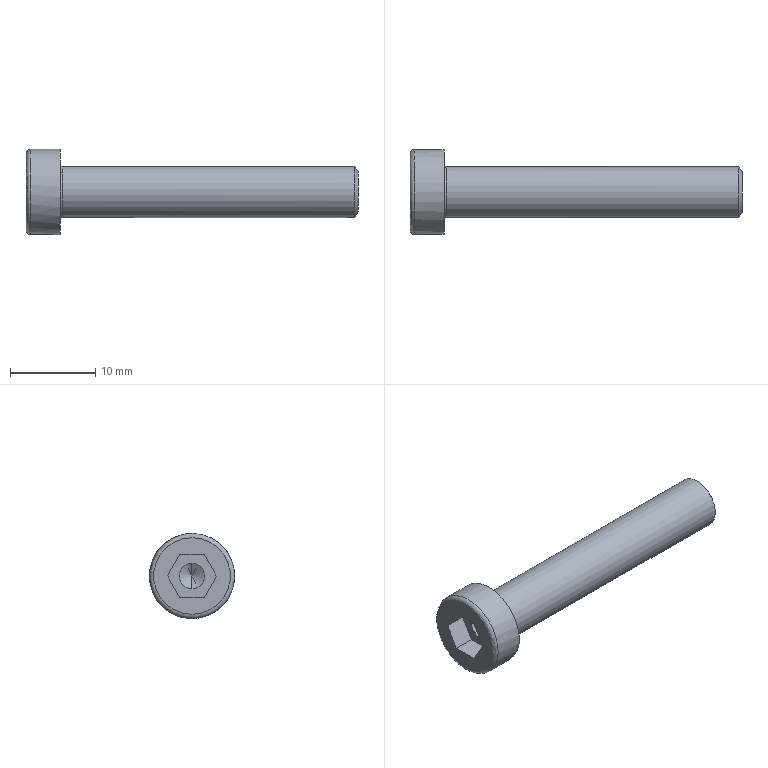Part | STEP file | Part [20] | 1 solid | 18 faces | box 39 x 10 x 10 mm | volume 1226 mm3 | plane 10 | cylinder 3 | cone 3 | torus 2 | commonest cylinder face diameters 3 x1 6 x1 10 x1
STEP:
#1=CARTESIAN_POINT('',(-20.293,107.5,4.5));
#2=VERTEX_POINT('',#1);
#3=CARTESIAN_POINT('',(-20.293,107.5,0.));
#4=DIRECTION('',(-1.,0.,0.));
#5=DIRECTION('',(0.,0.,1.));
#6=AXIS2_PLACEMENT_3D('',#3,#4,#5);
#7=CIRCLE('',#6,4.5);
#8=EDGE_CURVE('',#2,#2,#7,.T.);
#9=ORIENTED_EDGE('',*,*,#8,.T.);
#10=EDGE_LOOP('',(#9));
#11=FACE_BOUND('',#10,.T.);
#12=CARTESIAN_POINT('',(-20.293,108.948,-2.497));
#13=VERTEX_POINT('',#12);
#14=CARTESIAN_POINT('',(-20.293,110.387,0.005038));
#15=VERTEX_POINT('',#14);
#16=CARTESIAN_POINT('',(-20.293,108.948,-2.497));
#17=DIRECTION('',(0.,0.4985,0.8669));
#18=VECTOR('',#17,1.);
#19=LINE('',#16,#18);
#20=EDGE_CURVE('',#13,#15,#19,.T.);
#21=ORIENTED_EDGE('',*,*,#20,.T.);
#22=CARTESIAN_POINT('',(-20.293,108.939,2.503));
#23=VERTEX_POINT('',#22);
#24=CARTESIAN_POINT('',(-20.293,110.387,0.005038));
#25=DIRECTION('',(0.,-0.5015,0.8652));
#26=VECTOR('',#25,1.);
#27=LINE('',#24,#26);
#28=EDGE_CURVE('',#15,#23,#27,.T.);
#29=ORIENTED_EDGE('',*,*,#28,.T.);
#30=CARTESIAN_POINT('',(-20.293,106.052,2.497));
#31=VERTEX_POINT('',#30);
#32=CARTESIAN_POINT('',(-20.293,108.939,2.503));
#33=DIRECTION('',(0.,-1.,-0.001745));
#34=VECTOR('',#33,1.);
#35=LINE('',#32,#34);
#36=EDGE_CURVE('',#23,#31,#35,.T.);
#37=ORIENTED_EDGE('',*,*,#36,.T.);
#38=CARTESIAN_POINT('',(-20.293,104.613,-0.005038));
#39=VERTEX_POINT('',#38);
#40=CARTESIAN_POINT('',(-20.293,106.052,2.497));
#41=DIRECTION('',(0.,-0.4985,-0.8669));
#42=VECTOR('',#41,1.);
#43=LINE('',#40,#42);
#44=EDGE_CURVE('',#31,#39,#43,.T.);
#45=ORIENTED_EDGE('',*,*,#44,.T.);
#46=CARTESIAN_POINT('',(-20.293,106.061,-2.503));
#47=VERTEX_POINT('',#46);
#48=CARTESIAN_POINT('',(-20.293,104.613,-0.005038));
#49=DIRECTION('',(0.,0.5015,-0.8652));
#50=VECTOR('',#49,1.);
#51=LINE('',#48,#50);
#52=EDGE_CURVE('',#39,#47,#51,.T.);
#53=ORIENTED_EDGE('',*,*,#52,.T.);
#54=CARTESIAN_POINT('',(-20.293,106.061,-2.503));
#55=DIRECTION('',(0.,1.,0.001745));
#56=VECTOR('',#55,1.);
#57=LINE('',#54,#56);
#58=EDGE_CURVE('',#47,#13,#57,.T.);
#59=ORIENTED_EDGE('',*,*,#58,.T.);
#60=EDGE_LOOP('',(#21,#29,#37,#45,#53,#59));
#61=FACE_BOUND('',#60,.T.);
#62=CARTESIAN_POINT('',(-20.293,107.5,0.));
#63=DIRECTION('',(1.,0.,0.));
#64=DIRECTION('',(0.,0.,1.));
#65=AXIS2_PLACEMENT_3D('',#62,#63,#64);
#66=PLANE('',#65);
#67=ADVANCED_FACE('',(#11,#61),#66,.F.);
#68=CARTESIAN_POINT('',(-19.793,107.5,5.));
#69=VERTEX_POINT('',#68);
#70=CARTESIAN_POINT('',(-19.793,107.5,5.));
#71=CARTESIAN_POINT('',(-19.793,107.395,5.));
#72=CARTESIAN_POINT('',(-19.793,107.186,4.993));
#73=CARTESIAN_POINT('',(-19.793,106.873,4.964));
#74=CARTESIAN_POINT('',(-19.793,106.562,4.915));
#75=CARTESIAN_POINT('',(-19.793,106.256,4.846));
#76=CARTESIAN_POINT('',(-19.793,105.954,4.758));
#77=CARTESIAN_POINT('',(-19.793,105.658,4.652));
#78=CARTESIAN_POINT('',(-19.793,105.369,4.527));
#79=CARTESIAN_POINT('',(-19.793,105.089,4.384));
#80=CARTESIAN_POINT('',(-19.793,104.819,4.224));
#81=CARTESIAN_POINT('',(-19.793,104.559,4.047));
#82=CARTESIAN_POINT('',(-19.793,104.31,3.855));
#83=CARTESIAN_POINT('',(-19.793,104.075,3.647));
#84=CARTESIAN_POINT('',(-19.793,103.852,3.425));
#85=CARTESIAN_POINT('',(-19.793,103.644,3.189));
#86=CARTESIAN_POINT('',(-19.793,103.452,2.94));
#87=CARTESIAN_POINT('',(-19.793,103.275,2.68));
#88=CARTESIAN_POINT('',(-19.793,103.115,2.41));
#89=CARTESIAN_POINT('',(-19.793,102.973,2.129));
#90=CARTESIAN_POINT('',(-19.793,102.848,1.841));
#91=CARTESIAN_POINT('',(-19.793,102.741,1.545));
#92=CARTESIAN_POINT('',(-19.793,102.654,1.243));
#93=CARTESIAN_POINT('',(-19.793,102.585,0.9364));
#94=CARTESIAN_POINT('',(-19.793,102.536,0.6259));
#95=CARTESIAN_POINT('',(-19.793,102.507,0.313));
#96=CARTESIAN_POINT('',(-19.793,102.497,-0.001251));
#97=CARTESIAN_POINT('',(-19.793,102.507,-0.3155));
#98=CARTESIAN_POINT('',(-19.793,102.536,-0.6284));
#99=CARTESIAN_POINT('',(-19.793,102.586,-0.9389));
#100=CARTESIAN_POINT('',(-19.793,102.654,-1.246));
#101=CARTESIAN_POINT('',(-19.793,102.742,-1.548));
#102=CARTESIAN_POINT('',(-19.793,102.849,-1.843));
#103=CARTESIAN_POINT('',(-19.793,102.974,-2.132));
#104=CARTESIAN_POINT('',(-19.793,103.116,-2.412));
#105=CARTESIAN_POINT('',(-19.793,103.276,-2.682));
#106=CARTESIAN_POINT('',(-19.793,103.453,-2.942));
#107=CARTESIAN_POINT('',(-19.793,103.646,-3.191));
#108=CARTESIAN_POINT('',(-19.793,103.854,-3.426));
#109=CARTESIAN_POINT('',(-19.793,104.076,-3.649));
#110=CARTESIAN_POINT('',(-19.793,104.312,-3.856));
#111=CARTESIAN_POINT('',(-19.793,104.561,-4.049));
#112=CARTESIAN_POINT('',(-19.793,104.821,-4.226));
#113=CARTESIAN_POINT('',(-19.793,105.091,-4.385));
#114=CARTESIAN_POINT('',(-19.793,105.372,-4.528));
#115=CARTESIAN_POINT('',(-19.793,105.66,-4.653));
#116=CARTESIAN_POINT('',(-19.793,105.956,-4.759));
#117=CARTESIAN_POINT('',(-19.793,106.258,-4.847));
#118=CARTESIAN_POINT('',(-19.793,106.565,-4.915));
#119=CARTESIAN_POINT('',(-19.793,106.875,-4.964));
#120=CARTESIAN_POINT('',(-19.793,107.187,-4.993));
#121=CARTESIAN_POINT('',(-19.793,107.396,-5.));
#122=CARTESIAN_POINT('',(-19.793,107.5,-5.));
#123=CARTESIAN_POINT('',(-19.793,107.605,-5.));
#124=CARTESIAN_POINT('',(-19.793,107.814,-4.993));
#125=CARTESIAN_POINT('',(-19.793,108.127,-4.964));
#126=CARTESIAN_POINT('',(-19.793,108.438,-4.915));
#127=CARTESIAN_POINT('',(-19.793,108.744,-4.846));
#128=CARTESIAN_POINT('',(-19.793,109.046,-4.758));
#129=CARTESIAN_POINT('',(-19.793,109.342,-4.652));
#130=CARTESIAN_POINT('',(-19.793,109.631,-4.527));
#131=CARTESIAN_POINT('',(-19.793,109.911,-4.384));
#132=CARTESIAN_POINT('',(-19.793,110.181,-4.224));
#133=CARTESIAN_POINT('',(-19.793,110.441,-4.047));
#134=CARTESIAN_POINT('',(-19.793,110.69,-3.855));
#135=CARTESIAN_POINT('',(-19.793,110.925,-3.647));
#136=CARTESIAN_POINT('',(-19.793,111.148,-3.425));
#137=CARTESIAN_POINT('',(-19.793,111.356,-3.189));
#138=CARTESIAN_POINT('',(-19.793,111.548,-2.94));
#139=CARTESIAN_POINT('',(-19.793,111.725,-2.68));
#140=CARTESIAN_POINT('',(-19.793,111.885,-2.41));
#141=CARTESIAN_POINT('',(-19.793,112.027,-2.129));
#142=CARTESIAN_POINT('',(-19.793,112.152,-1.841));
#143=CARTESIAN_POINT('',(-19.793,112.259,-1.545));
#144=CARTESIAN_POINT('',(-19.793,112.346,-1.243));
#145=CARTESIAN_POINT('',(-19.793,112.415,-0.9364));
#146=CARTESIAN_POINT('',(-19.793,112.464,-0.6259));
#147=CARTESIAN_POINT('',(-19.793,112.493,-0.313));
#148=CARTESIAN_POINT('',(-19.793,112.503,0.001251));
#149=CARTESIAN_POINT('',(-19.793,112.493,0.3155));
#150=CARTESIAN_POINT('',(-19.793,112.464,0.6284));
#151=CARTESIAN_POINT('',(-19.793,112.414,0.9389));
#152=CARTESIAN_POINT('',(-19.793,112.346,1.246));
#153=CARTESIAN_POINT('',(-19.793,112.258,1.548));
#154=CARTESIAN_POINT('',(-19.793,112.151,1.843));
#155=CARTESIAN_POINT('',(-19.793,112.026,2.132));
#156=CARTESIAN_POINT('',(-19.793,111.884,2.412));
#157=CARTESIAN_POINT('',(-19.793,111.724,2.682));
#158=CARTESIAN_POINT('',(-19.793,111.547,2.942));
#159=CARTESIAN_POINT('',(-19.793,111.354,3.191));
#160=CARTESIAN_POINT('',(-19.793,111.146,3.426));
#161=CARTESIAN_POINT('',(-19.793,110.924,3.649));
#162=CARTESIAN_POINT('',(-19.793,110.688,3.856));
#163=CARTESIAN_POINT('',(-19.793,110.439,4.049));
#164=CARTESIAN_POINT('',(-19.793,110.179,4.226));
#165=CARTESIAN_POINT('',(-19.793,109.909,4.385));
#166=CARTESIAN_POINT('',(-19.793,109.628,4.528));
#167=CARTESIAN_POINT('',(-19.793,109.34,4.653));
#168=CARTESIAN_POINT('',(-19.793,109.044,4.759));
#169=CARTESIAN_POINT('',(-19.793,108.742,4.847));
#170=CARTESIAN_POINT('',(-19.793,108.435,4.915));
#171=CARTESIAN_POINT('',(-19.793,108.125,4.964));
#172=CARTESIAN_POINT('',(-19.793,107.813,4.993));
#173=CARTESIAN_POINT('',(-19.793,107.604,5.));
#174=CARTESIAN_POINT('',(-19.793,107.5,5.));
#175=B_SPLINE_CURVE_WITH_KNOTS('',3,(#70,#71,#72,#73,#74,#75,#76,#77,#78,#79,#80,#81,#82,#83,#84,#85,#86,#87,#88,#89,#90,#91,#92,#93,#94,#95,#96,#97,#98,#99,#100,#101,#102,#103,#104,#105,#106,#107,#108,#109,#110,#111,#112,#113,#114,#115,#116,#117,#118,#119,#120,#121,#122,#123,#124,#125,#126,#127,#128,#129,#130,#131,#132,#133,#134,#135,#136,#137,#138,#139,#140,#141,#142,#143,#144,#145,#146,#147,#148,#149,#150,#151,#152,#153,#154,#155,#156,#157,#158,#159,#160,#161,#162,#163,#164,#165,#166,#167,#168,#169,#170,#171,#172,#173,#174),.UNSPECIFIED.,.T.,.F.,(4,1,1,1,1,1,1,1,1,1,1,1,1,1,1,1,1,1,1,1,1,1,1,1,1,1,1,1,1,1,1,1,1,1,1,1,1,1,1,1,1,1,1,1,1,1,1,1,1,1,3,1,1,1,1,1,1,1,1,1,1,1,1,1,1,1,1,1,1,1,1,1,1,1,1,1,1,1,1,1,1,1,1,1,1,1,1,1,1,1,1,1,1,1,1,1,1,1,1,1,4),(0.,0.01,0.02,0.03,0.04001,0.05001,0.06001,0.07001,0.08001,0.09001,0.1,0.11,0.12,0.13,0.14,0.15,0.16,0.17,0.18,0.19,0.2,0.21,0.22,0.23,0.24,0.25,0.26,0.27,0.28,0.29,0.3,0.31,0.3201,0.3301,0.3401,0.3501,0.3601,0.3701,0.3801,0.3901,0.4001,0.4101,0.4201,0.4301,0.4401,0.4501,0.4601,0.4701,0.4801,0.4901,0.5,0.51,0.52,0.53,0.54,0.55,0.56,0.57,0.58,0.59,0.6,0.61,0.62,0.63,0.64,0.65,0.66,0.67,0.68,0.69,0.7,0.71,0.72,0.73,0.74,0.75,0.76,0.77,0.78,0.79,0.8,0.81,0.8201,0.8301,0.8401,0.8501,0.8601,0.8701,0.8801,0.8901,0.9001,0.9101,0.9201,0.9301,0.9401,0.9501,0.9601,0.9701,0.9801,0.9901,1.),.UNSPECIFIED.);
#176=EDGE_CURVE('',#69,#69,#175,.T.);
#177=ORIENTED_EDGE('',*,*,#176,.F.);
#178=EDGE_LOOP('',(#177));
#179=FACE_OUTER_BOUND('',#178,.T.);
#180=ORIENTED_EDGE('',*,*,#8,.F.);
#181=EDGE_LOOP('',(#180));
#182=FACE_OUTER_BOUND('',#181,.T.);
#183=CARTESIAN_POINT('',(-19.793,107.5,0.));
#184=DIRECTION('',(1.,0.,0.));
#185=DIRECTION('',(0.,0.,1.));
#186=AXIS2_PLACEMENT_3D('',#183,#184,#185);
#187=TOROIDAL_SURFACE('',#186,4.5,0.5);
#188=ADVANCED_FACE('',(#179,#182),#187,.T.);
#189=CARTESIAN_POINT('',(-16.293,107.5,5.));
#190=VERTEX_POINT('',#189);
#191=CARTESIAN_POINT('',(-16.293,107.5,0.));
#192=DIRECTION('',(1.,0.,0.));
#193=DIRECTION('',(0.,0.,1.));
#194=AXIS2_PLACEMENT_3D('',#191,#192,#193);
#195=CIRCLE('',#194,5.);
#196=EDGE_CURVE('',#190,#190,#195,.T.);
#197=ORIENTED_EDGE('',*,*,#196,.F.);
#198=EDGE_LOOP('',(#197));
#199=FACE_OUTER_BOUND('',#198,.T.);
#200=ORIENTED_EDGE('',*,*,#176,.T.);
#201=EDGE_LOOP('',(#200));
#202=FACE_OUTER_BOUND('',#201,.T.);
#203=CARTESIAN_POINT('',(-22.243,107.5,0.));
#204=DIRECTION('',(1.,0.,0.));
#205=DIRECTION('',(0.,0.,1.));
#206=AXIS2_PLACEMENT_3D('',#203,#204,#205);
#207=CYLINDRICAL_SURFACE('',#206,5.);
#208=ADVANCED_FACE('',(#199,#202),#207,.T.);
#209=ORIENTED_EDGE('',*,*,#196,.T.);
#210=EDGE_LOOP('',(#209));
#211=FACE_BOUND('',#210,.T.);
#212=CARTESIAN_POINT('',(-16.293,107.5,3.25));
#213=VERTEX_POINT('',#212);
#214=CARTESIAN_POINT('',(-16.293,107.5,0.));
#215=DIRECTION('',(1.,0.,0.));
#216=DIRECTION('',(0.,0.,1.));
#217=AXIS2_PLACEMENT_3D('',#214,#215,#216);
#218=CIRCLE('',#217,3.25);
#219=EDGE_CURVE('',#213,#213,#218,.T.);
#220=ORIENTED_EDGE('',*,*,#219,.F.);
#221=EDGE_LOOP('',(#220));
#222=FACE_BOUND('',#221,.T.);
#223=CARTESIAN_POINT('',(-16.293,107.5,0.));
#224=DIRECTION('',(1.,0.,0.));
#225=DIRECTION('',(0.,0.,1.));
#226=AXIS2_PLACEMENT_3D('',#223,#224,#225);
#227=PLANE('',#226);
#228=ADVANCED_FACE('',(#211,#222),#227,.T.);
#229=CARTESIAN_POINT('',(-16.043,107.5,3.));
#230=VERTEX_POINT('',#229);
#231=CARTESIAN_POINT('',(-16.043,107.5,3.));
#232=CARTESIAN_POINT('',(-16.043,107.437,3.));
#233=CARTESIAN_POINT('',(-16.043,107.311,2.996));
#234=CARTESIAN_POINT('',(-16.043,107.124,2.978));
#235=CARTESIAN_POINT('',(-16.043,106.937,2.949));
#236=CARTESIAN_POINT('',(-16.043,106.753,2.908));
#237=CARTESIAN_POINT('',(-16.043,106.572,2.855));
#238=CARTESIAN_POINT('',(-16.043,106.395,2.791));
#239=CARTESIAN_POINT('',(-16.043,106.222,2.716));
#240=CARTESIAN_POINT('',(-16.043,106.054,2.631));
#241=CARTESIAN_POINT('',(-16.043,105.891,2.535));
#242=CARTESIAN_POINT('',(-16.043,105.735,2.428));
#243=CARTESIAN_POINT('',(-16.043,105.586,2.313));
#244=CARTESIAN_POINT('',(-16.043,105.445,2.188));
#245=CARTESIAN_POINT('',(-16.043,105.311,2.055));
#246=CARTESIAN_POINT('',(-16.043,105.187,1.913));
#247=CARTESIAN_POINT('',(-16.043,105.071,1.764));
#248=CARTESIAN_POINT('',(-16.043,104.965,1.608));
#249=CARTESIAN_POINT('',(-16.043,104.869,1.446));
#250=CARTESIAN_POINT('',(-16.043,104.784,1.278));
#251=CARTESIAN_POINT('',(-16.043,104.709,1.105));
#252=CARTESIAN_POINT('',(-16.043,104.645,0.9271));
#253=CARTESIAN_POINT('',(-16.043,104.592,0.746));
#254=CARTESIAN_POINT('',(-16.043,104.551,0.5619));
#255=CARTESIAN_POINT('',(-16.043,104.522,0.3756));
#256=CARTESIAN_POINT('',(-16.043,104.504,0.1878));
#257=CARTESIAN_POINT('',(-16.043,104.498,-0.0007505));
#258=CARTESIAN_POINT('',(-16.043,104.504,-0.1893));
#259=CARTESIAN_POINT('',(-16.043,104.522,-0.3771));
#260=CARTESIAN_POINT('',(-16.043,104.551,-0.5633));
#261=CARTESIAN_POINT('',(-16.043,104.593,-0.7474));
#262=CARTESIAN_POINT('',(-16.043,104.645,-0.9285));
#263=CARTESIAN_POINT('',(-16.043,104.709,-1.106));
#264=CARTESIAN_POINT('',(-16.043,104.784,-1.279));
#265=CARTESIAN_POINT('',(-16.043,104.87,-1.447));
#266=CARTESIAN_POINT('',(-16.043,104.966,-1.609));
#267=CARTESIAN_POINT('',(-16.043,105.072,-1.765));
#268=CARTESIAN_POINT('',(-16.043,105.188,-1.914));
#269=CARTESIAN_POINT('',(-16.043,105.312,-2.056));
#270=CARTESIAN_POINT('',(-16.043,105.446,-2.189));
#271=CARTESIAN_POINT('',(-16.043,105.587,-2.314));
#272=CARTESIAN_POINT('',(-16.043,105.736,-2.429));
#273=CARTESIAN_POINT('',(-16.043,105.893,-2.535));
#274=CARTESIAN_POINT('',(-16.043,106.055,-2.631));
#275=CARTESIAN_POINT('',(-16.043,106.223,-2.717));
#276=CARTESIAN_POINT('',(-16.043,106.396,-2.792));
#277=CARTESIAN_POINT('',(-16.043,106.574,-2.855));
#278=CARTESIAN_POINT('',(-16.043,106.755,-2.908));
#279=CARTESIAN_POINT('',(-16.043,106.939,-2.949));
#280=CARTESIAN_POINT('',(-16.043,107.125,-2.978));
#281=CARTESIAN_POINT('',(-16.043,107.312,-2.996));
#282=CARTESIAN_POINT('',(-16.043,107.438,-3.));
#283=CARTESIAN_POINT('',(-16.043,107.5,-3.));
#284=CARTESIAN_POINT('',(-16.043,107.563,-3.));
#285=CARTESIAN_POINT('',(-16.043,107.689,-2.996));
#286=CARTESIAN_POINT('',(-16.043,107.876,-2.978));
#287=CARTESIAN_POINT('',(-16.043,108.063,-2.949));
#288=CARTESIAN_POINT('',(-16.043,108.247,-2.908));
#289=CARTESIAN_POINT('',(-16.043,108.428,-2.855));
#290=CARTESIAN_POINT('',(-16.043,108.605,-2.791));
#291=CARTESIAN_POINT('',(-16.043,108.778,-2.716));
#292=CARTESIAN_POINT('',(-16.043,108.946,-2.631));
#293=CARTESIAN_POINT('',(-16.043,109.109,-2.535));
#294=CARTESIAN_POINT('',(-16.043,109.265,-2.428));
#295=CARTESIAN_POINT('',(-16.043,109.414,-2.313));
#296=CARTESIAN_POINT('',(-16.043,109.555,-2.188));
#297=CARTESIAN_POINT('',(-16.043,109.689,-2.055));
#298=CARTESIAN_POINT('',(-16.043,109.813,-1.913));
#299=CARTESIAN_POINT('',(-16.043,109.929,-1.764));
#300=CARTESIAN_POINT('',(-16.043,110.035,-1.608));
#301=CARTESIAN_POINT('',(-16.043,110.131,-1.446));
#302=CARTESIAN_POINT('',(-16.043,110.216,-1.278));
#303=CARTESIAN_POINT('',(-16.043,110.291,-1.105));
#304=CARTESIAN_POINT('',(-16.043,110.355,-0.9271));
#305=CARTESIAN_POINT('',(-16.043,110.408,-0.746));
#306=CARTESIAN_POINT('',(-16.043,110.449,-0.5619));
#307=CARTESIAN_POINT('',(-16.043,110.478,-0.3756));
#308=CARTESIAN_POINT('',(-16.043,110.496,-0.1878));
#309=CARTESIAN_POINT('',(-16.043,110.502,0.0007505));
#310=CARTESIAN_POINT('',(-16.043,110.496,0.1893));
#311=CARTESIAN_POINT('',(-16.043,110.478,0.3771));
#312=CARTESIAN_POINT('',(-16.043,110.449,0.5633));
#313=CARTESIAN_POINT('',(-16.043,110.407,0.7474));
#314=CARTESIAN_POINT('',(-16.043,110.355,0.9285));
#315=CARTESIAN_POINT('',(-16.043,110.291,1.106));
#316=CARTESIAN_POINT('',(-16.043,110.216,1.279));
#317=CARTESIAN_POINT('',(-16.043,110.13,1.447));
#318=CARTESIAN_POINT('',(-16.043,110.034,1.609));
#319=CARTESIAN_POINT('',(-16.043,109.928,1.765));
#320=CARTESIAN_POINT('',(-16.043,109.812,1.914));
#321=CARTESIAN_POINT('',(-16.043,109.688,2.056));
#322=CARTESIAN_POINT('',(-16.043,109.554,2.189));
#323=CARTESIAN_POINT('',(-16.043,109.413,2.314));
#324=CARTESIAN_POINT('',(-16.043,109.264,2.429));
#325=CARTESIAN_POINT('',(-16.043,109.107,2.535));
#326=CARTESIAN_POINT('',(-16.043,108.945,2.631));
#327=CARTESIAN_POINT('',(-16.043,108.777,2.717));
#328=CARTESIAN_POINT('',(-16.043,108.604,2.792));
#329=CARTESIAN_POINT('',(-16.043,108.426,2.855));
#330=CARTESIAN_POINT('',(-16.043,108.245,2.908));
#331=CARTESIAN_POINT('',(-16.043,108.061,2.949));
#332=CARTESIAN_POINT('',(-16.043,107.875,2.978));
#333=CARTESIAN_POINT('',(-16.043,107.688,2.996));
#334=CARTESIAN_POINT('',(-16.043,107.562,3.));
#335=CARTESIAN_POINT('',(-16.043,107.5,3.));
#336=B_SPLINE_CURVE_WITH_KNOTS('',3,(#231,#232,#233,#234,#235,#236,#237,#238,#239,#240,#241,#242,#243,#244,#245,#246,#247,#248,#249,#250,#251,#252,#253,#254,#255,#256,#257,#258,#259,#260,#261,#262,#263,#264,#265,#266,#267,#268,#269,#270,#271,#272,#273,#274,#275,#276,#277,#278,#279,#280,#281,#282,#283,#284,#285,#286,#287,#288,#289,#290,#291,#292,#293,#294,#295,#296,#297,#298,#299,#300,#301,#302,#303,#304,#305,#306,#307,#308,#309,#310,#311,#312,#313,#314,#315,#316,#317,#318,#319,#320,#321,#322,#323,#324,#325,#326,#327,#328,#329,#330,#331,#332,#333,#334,#335),.UNSPECIFIED.,.T.,.F.,(4,1,1,1,1,1,1,1,1,1,1,1,1,1,1,1,1,1,1,1,1,1,1,1,1,1,1,1,1,1,1,1,1,1,1,1,1,1,1,1,1,1,1,1,1,1,1,1,1,1,3,1,1,1,1,1,1,1,1,1,1,1,1,1,1,1,1,1,1,1,1,1,1,1,1,1,1,1,1,1,1,1,1,1,1,1,1,1,1,1,1,1,1,1,1,1,1,1,1,1,4),(0.,0.01,0.02,0.03,0.04001,0.05001,0.06001,0.07001,0.08001,0.09001,0.1,0.11,0.12,0.13,0.14,0.15,0.16,0.17,0.18,0.19,0.2,0.21,0.22,0.23,0.24,0.25,0.26,0.27,0.28,0.29,0.3,0.31,0.3201,0.3301,0.3401,0.3501,0.3601,0.3701,0.3801,0.3901,0.4001,0.4101,0.4201,0.4301,0.4401,0.4501,0.4601,0.4701,0.4801,0.4901,0.5,0.51,0.52,0.53,0.54,0.55,0.56,0.57,0.58,0.59,0.6,0.61,0.62,0.63,0.64,0.65,0.66,0.67,0.68,0.69,0.7,0.71,0.72,0.73,0.74,0.75,0.76,0.77,0.78,0.79,0.8,0.81,0.8201,0.8301,0.8401,0.8501,0.8601,0.8701,0.8801,0.8901,0.9001,0.9101,0.9201,0.9301,0.9401,0.9501,0.9601,0.9701,0.9801,0.9901,1.),.UNSPECIFIED.);
#337=EDGE_CURVE('',#230,#230,#336,.T.);
#338=ORIENTED_EDGE('',*,*,#337,.F.);
#339=EDGE_LOOP('',(#338));
#340=FACE_OUTER_BOUND('',#339,.T.);
#341=ORIENTED_EDGE('',*,*,#219,.T.);
#342=EDGE_LOOP('',(#341));
#343=FACE_OUTER_BOUND('',#342,.T.);
#344=CARTESIAN_POINT('',(-16.043,107.5,0.));
#345=DIRECTION('',(1.,0.,0.));
#346=DIRECTION('',(0.,0.,1.));
#347=AXIS2_PLACEMENT_3D('',#344,#345,#346);
#348=TOROIDAL_SURFACE('',#347,3.25,0.25);
#349=ADVANCED_FACE('',(#340,#343),#348,.F.);
#350=CARTESIAN_POINT('',(18.273,107.5,3.));
#351=VERTEX_POINT('',#350);
#352=CARTESIAN_POINT('',(18.273,107.5,-3.));
#353=VERTEX_POINT('',#352);
#354=CARTESIAN_POINT('',(18.273,107.5,0.));
#355=DIRECTION('',(-1.,0.,0.));
#356=DIRECTION('',(0.,0.,1.));
#357=AXIS2_PLACEMENT_3D('',#354,#355,#356);
#358=CIRCLE('',#357,3.);
#359=EDGE_CURVE('',#351,#353,#358,.T.);
#360=ORIENTED_EDGE('',*,*,#359,.T.);
#361=CARTESIAN_POINT('',(18.273,107.5,0.));
#362=DIRECTION('',(1.,0.,0.));
#363=DIRECTION('',(0.,0.,1.));
#364=AXIS2_PLACEMENT_3D('',#361,#362,#363);
#365=CIRCLE('',#364,3.);
#366=EDGE_CURVE('',#351,#353,#365,.T.);
#367=ORIENTED_EDGE('',*,*,#366,.F.);
#368=EDGE_LOOP('',(#360,#367));
#369=FACE_BOUND('',#368,.T.);
#370=ORIENTED_EDGE('',*,*,#337,.T.);
#371=EDGE_LOOP('',(#370));
#372=FACE_OUTER_BOUND('',#371,.T.);
#373=CARTESIAN_POINT('',(-22.243,107.5,0.));
#374=DIRECTION('',(1.,0.,0.));
#375=DIRECTION('',(0.,0.,1.));
#376=AXIS2_PLACEMENT_3D('',#373,#374,#375);
#377=CYLINDRICAL_SURFACE('',#376,3.);
#378=ADVANCED_FACE('',(#369,#372),#377,.T.);
#379=CARTESIAN_POINT('',(18.707,107.5,-2.386));
#380=VERTEX_POINT('',#379);
#381=CARTESIAN_POINT('',(18.707,107.5,0.));
#382=DIRECTION('',(1.,0.,0.));
#383=DIRECTION('',(0.,0.,1.));
#384=AXIS2_PLACEMENT_3D('',#381,#382,#383);
#385=CIRCLE('',#384,2.386);
#386=EDGE_CURVE('',#380,#380,#385,.T.);
#387=ORIENTED_EDGE('',*,*,#386,.F.);
#388=EDGE_LOOP('',(#387));
#389=FACE_OUTER_BOUND('',#388,.T.);
#390=ORIENTED_EDGE('',*,*,#366,.T.);
#391=ORIENTED_EDGE('',*,*,#359,.F.);
#392=EDGE_LOOP('',(#390,#391));
#393=FACE_BOUND('',#392,.T.);
#394=CARTESIAN_POINT('',(18.49,107.5,0.));
#395=DIRECTION('',(-1.,0.,0.));
#396=DIRECTION('',(0.,0.,-1.));
#397=AXIS2_PLACEMENT_3D('',#394,#395,#396);
#398=CONICAL_SURFACE('',#397,2.693,0.9553);
#399=ADVANCED_FACE('',(#389,#393),#398,.T.);
#400=ORIENTED_EDGE('',*,*,#386,.T.);
#401=EDGE_LOOP('',(#400));
#402=FACE_BOUND('',#401,.T.);
#403=CARTESIAN_POINT('',(18.707,107.5,0.));
#404=DIRECTION('',(1.,0.,0.));
#405=DIRECTION('',(0.,0.,1.));
#406=AXIS2_PLACEMENT_3D('',#403,#404,#405);
#407=PLANE('',#406);
#408=ADVANCED_FACE('',(#402),#407,.T.);
#409=CARTESIAN_POINT('',(-17.793,106.061,-2.503));
#410=VERTEX_POINT('',#409);
#411=CARTESIAN_POINT('',(-17.793,106.061,-2.503));
#412=DIRECTION('',(-1.,0.,0.));
#413=VECTOR('',#412,1.);
#414=LINE('',#411,#413);
#415=EDGE_CURVE('',#410,#47,#414,.T.);
#416=ORIENTED_EDGE('',*,*,#415,.F.);
#417=CARTESIAN_POINT('',(-17.793,108.948,-2.497));
#418=VERTEX_POINT('',#417);
#419=CARTESIAN_POINT('',(-17.793,106.061,-2.503));
#420=DIRECTION('',(0.,1.,0.001745));
#421=VECTOR('',#420,1.);
#422=LINE('',#419,#421);
#423=EDGE_CURVE('',#410,#418,#422,.T.);
#424=ORIENTED_EDGE('',*,*,#423,.T.);
#425=CARTESIAN_POINT('',(-17.793,108.948,-2.497));
#426=DIRECTION('',(-1.,0.,0.));
#427=VECTOR('',#426,1.);
#428=LINE('',#425,#427);
#429=EDGE_CURVE('',#418,#13,#428,.T.);
#430=ORIENTED_EDGE('',*,*,#429,.T.);
#431=ORIENTED_EDGE('',*,*,#58,.F.);
#432=EDGE_LOOP('',(#416,#424,#430,#431));
#433=FACE_BOUND('',#432,.T.);
#434=CARTESIAN_POINT('',(-17.793,106.061,-2.503));
#435=DIRECTION('',(0.,0.001745,-1.));
#436=DIRECTION('',(-1.,0.,0.));
#437=AXIS2_PLACEMENT_3D('',#434,#435,#436);
#438=PLANE('',#437);
#439=ADVANCED_FACE('',(#433),#438,.F.);
#440=ORIENTED_EDGE('',*,*,#429,.F.);
#441=CARTESIAN_POINT('',(-17.793,110.387,0.005038));
#442=VERTEX_POINT('',#441);
#443=CARTESIAN_POINT('',(-17.793,108.948,-2.497));
#444=DIRECTION('',(0.,0.4985,0.8669));
#445=VECTOR('',#444,1.);
#446=LINE('',#443,#445);
#447=EDGE_CURVE('',#418,#442,#446,.T.);
#448=ORIENTED_EDGE('',*,*,#447,.T.);
#449=CARTESIAN_POINT('',(-17.793,110.387,0.005038));
#450=DIRECTION('',(-1.,0.,0.));
#451=VECTOR('',#450,1.);
#452=LINE('',#449,#451);
#453=EDGE_CURVE('',#442,#15,#452,.T.);
#454=ORIENTED_EDGE('',*,*,#453,.T.);
#455=ORIENTED_EDGE('',*,*,#20,.F.);
#456=EDGE_LOOP('',(#440,#448,#454,#455));
#457=FACE_BOUND('',#456,.T.);
#458=CARTESIAN_POINT('',(-17.793,108.948,-2.497));
#459=DIRECTION('',(0.,0.8669,-0.4985));
#460=DIRECTION('',(-1.,0.,0.));
#461=AXIS2_PLACEMENT_3D('',#458,#459,#460);
#462=PLANE('',#461);
#463=ADVANCED_FACE('',(#457),#462,.F.);
#464=ORIENTED_EDGE('',*,*,#453,.F.);
#465=CARTESIAN_POINT('',(-17.793,108.939,2.503));
#466=VERTEX_POINT('',#465);
#467=CARTESIAN_POINT('',(-17.793,110.387,0.005038));
#468=DIRECTION('',(0.,-0.5015,0.8652));
#469=VECTOR('',#468,1.);
#470=LINE('',#467,#469);
#471=EDGE_CURVE('',#442,#466,#470,.T.);
#472=ORIENTED_EDGE('',*,*,#471,.T.);
#473=CARTESIAN_POINT('',(-17.793,108.939,2.503));
#474=DIRECTION('',(-1.,0.,0.));
#475=VECTOR('',#474,1.);
#476=LINE('',#473,#475);
#477=EDGE_CURVE('',#466,#23,#476,.T.);
#478=ORIENTED_EDGE('',*,*,#477,.T.);
#479=ORIENTED_EDGE('',*,*,#28,.F.);
#480=EDGE_LOOP('',(#464,#472,#478,#479));
#481=FACE_BOUND('',#480,.T.);
#482=CARTESIAN_POINT('',(-17.793,110.387,0.005038));
#483=DIRECTION('',(0.,0.8652,0.5015));
#484=DIRECTION('',(1.,0.,0.));
#485=AXIS2_PLACEMENT_3D('',#482,#483,#484);
#486=PLANE('',#485);
#487=ADVANCED_FACE('',(#481),#486,.F.);
#488=ORIENTED_EDGE('',*,*,#477,.F.);
#489=CARTESIAN_POINT('',(-17.793,106.052,2.497));
#490=VERTEX_POINT('',#489);
#491=CARTESIAN_POINT('',(-17.793,108.939,2.503));
#492=DIRECTION('',(0.,-1.,-0.001745));
#493=VECTOR('',#492,1.);
#494=LINE('',#491,#493);
#495=EDGE_CURVE('',#466,#490,#494,.T.);
#496=ORIENTED_EDGE('',*,*,#495,.T.);
#497=CARTESIAN_POINT('',(-17.793,106.052,2.497));
#498=DIRECTION('',(-1.,0.,0.));
#499=VECTOR('',#498,1.);
#500=LINE('',#497,#499);
#501=EDGE_CURVE('',#490,#31,#500,.T.);
#502=ORIENTED_EDGE('',*,*,#501,.T.);
#503=ORIENTED_EDGE('',*,*,#36,.F.);
#504=EDGE_LOOP('',(#488,#496,#502,#503));
#505=FACE_BOUND('',#504,.T.);
#506=CARTESIAN_POINT('',(-17.793,108.939,2.503));
#507=DIRECTION('',(0.,-0.001745,1.));
#508=DIRECTION('',(-1.,0.,0.));
#509=AXIS2_PLACEMENT_3D('',#506,#507,#508);
#510=PLANE('',#509);
#511=ADVANCED_FACE('',(#505),#510,.F.);
#512=ORIENTED_EDGE('',*,*,#501,.F.);
#513=CARTESIAN_POINT('',(-17.793,104.613,-0.005038));
#514=VERTEX_POINT('',#513);
#515=CARTESIAN_POINT('',(-17.793,106.052,2.497));
#516=DIRECTION('',(0.,-0.4985,-0.8669));
#517=VECTOR('',#516,1.);
#518=LINE('',#515,#517);
#519=EDGE_CURVE('',#490,#514,#518,.T.);
#520=ORIENTED_EDGE('',*,*,#519,.T.);
#521=CARTESIAN_POINT('',(-17.793,104.613,-0.005038));
#522=DIRECTION('',(-1.,0.,0.));
#523=VECTOR('',#522,1.);
#524=LINE('',#521,#523);
#525=EDGE_CURVE('',#514,#39,#524,.T.);
#526=ORIENTED_EDGE('',*,*,#525,.T.);
#527=ORIENTED_EDGE('',*,*,#44,.F.);
#528=EDGE_LOOP('',(#512,#520,#526,#527));
#529=FACE_BOUND('',#528,.T.);
#530=CARTESIAN_POINT('',(-17.793,106.052,2.497));
#531=DIRECTION('',(0.,-0.8669,0.4985));
#532=DIRECTION('',(-1.,0.,0.));
#533=AXIS2_PLACEMENT_3D('',#530,#531,#532);
#534=PLANE('',#533);
#535=ADVANCED_FACE('',(#529),#534,.F.);
#536=ORIENTED_EDGE('',*,*,#525,.F.);
#537=CARTESIAN_POINT('',(-17.793,104.613,-0.005038));
#538=DIRECTION('',(0.,0.5015,-0.8652));
#539=VECTOR('',#538,1.);
#540=LINE('',#537,#539);
#541=EDGE_CURVE('',#514,#410,#540,.T.);
#542=ORIENTED_EDGE('',*,*,#541,.T.);
#543=ORIENTED_EDGE('',*,*,#415,.T.);
#544=ORIENTED_EDGE('',*,*,#52,.F.);
#545=EDGE_LOOP('',(#536,#542,#543,#544));
#546=FACE_BOUND('',#545,.T.);
#547=CARTESIAN_POINT('',(-17.793,104.613,-0.005038));
#548=DIRECTION('',(0.,-0.8652,-0.5015));
#549=DIRECTION('',(0.,0.5015,-0.8652));
#550=AXIS2_PLACEMENT_3D('',#547,#548,#549);
#551=PLANE('',#550);
#552=ADVANCED_FACE('',(#546),#551,.F.);
#553=ORIENTED_EDGE('',*,*,#541,.F.);
#554=ORIENTED_EDGE('',*,*,#519,.F.);
#555=ORIENTED_EDGE('',*,*,#495,.F.);
#556=ORIENTED_EDGE('',*,*,#471,.F.);
#557=ORIENTED_EDGE('',*,*,#447,.F.);
#558=ORIENTED_EDGE('',*,*,#423,.F.);
#559=EDGE_LOOP('',(#553,#554,#555,#556,#557,#558));
#560=FACE_BOUND('',#559,.T.);
#561=CARTESIAN_POINT('',(-17.793,107.5,1.5));
#562=VERTEX_POINT('',#561);
#563=CARTESIAN_POINT('',(-17.793,107.5,0.));
#564=DIRECTION('',(1.,0.,0.));
#565=DIRECTION('',(0.,0.,1.));
#566=AXIS2_PLACEMENT_3D('',#563,#564,#565);
#567=CIRCLE('',#566,1.5);
#568=EDGE_CURVE('',#562,#562,#567,.T.);
#569=ORIENTED_EDGE('',*,*,#568,.T.);
#570=EDGE_LOOP('',(#569));
#571=FACE_BOUND('',#570,.T.);
#572=CARTESIAN_POINT('',(-17.793,107.5,0.));
#573=DIRECTION('',(1.,0.,0.));
#574=DIRECTION('',(0.,0.,1.));
#575=AXIS2_PLACEMENT_3D('',#572,#573,#574);
#576=PLANE('',#575);
#577=ADVANCED_FACE('',(#560,#571),#576,.F.);
#578=CARTESIAN_POINT('',(-15.293,107.5,1.5));
#579=VERTEX_POINT('',#578);
#580=CARTESIAN_POINT('',(-15.293,107.5,-1.5));
#581=VERTEX_POINT('',#580);
#582=CARTESIAN_POINT('',(-15.293,107.5,0.));
#583=DIRECTION('',(1.,0.,0.));
#584=DIRECTION('',(0.,0.,1.));
#585=AXIS2_PLACEMENT_3D('',#582,#583,#584);
#586=CIRCLE('',#585,1.5);
#587=EDGE_CURVE('',#579,#581,#586,.T.);
#588=ORIENTED_EDGE('',*,*,#587,.T.);
#589=CARTESIAN_POINT('',(-15.293,107.5,0.));
#590=DIRECTION('',(-1.,0.,0.));
#591=DIRECTION('',(0.,0.,1.));
#592=AXIS2_PLACEMENT_3D('',#589,#590,#591);
#593=CIRCLE('',#592,1.5);
#594=EDGE_CURVE('',#579,#581,#593,.T.);
#595=ORIENTED_EDGE('',*,*,#594,.F.);
#596=EDGE_LOOP('',(#588,#595));
#597=FACE_BOUND('',#596,.T.);
#598=ORIENTED_EDGE('',*,*,#568,.F.);
#599=EDGE_LOOP('',(#598));
#600=FACE_OUTER_BOUND('',#599,.T.);
#601=CARTESIAN_POINT('',(-20.586,107.5,0.));
#602=DIRECTION('',(1.,0.,0.));
#603=DIRECTION('',(0.,0.,1.));
#604=AXIS2_PLACEMENT_3D('',#601,#602,#603);
#605=CYLINDRICAL_SURFACE('',#604,1.5);
#606=ADVANCED_FACE('',(#597,#600),#605,.F.);
#607=CARTESIAN_POINT('',(-14.427,107.5,0.));
#608=VERTEX_POINT('',#607);
#609=CARTESIAN_POINT('',(-15.293,107.5,1.5));
#610=DIRECTION('',(0.5,0.,-0.866));
#611=VECTOR('',#610,1.);
#612=LINE('',#609,#611);
#613=EDGE_CURVE('',#579,#608,#612,.T.);
#614=ORIENTED_EDGE('',*,*,#613,.F.);
#615=ORIENTED_EDGE('',*,*,#594,.T.);
#616=CARTESIAN_POINT('',(-15.293,107.5,-1.5));
#617=DIRECTION('',(0.5,0.,0.866));
#618=VECTOR('',#617,1.);
#619=LINE('',#616,#618);
#620=EDGE_CURVE('',#581,#608,#619,.T.);
#621=ORIENTED_EDGE('',*,*,#620,.T.);
#622=EDGE_LOOP('',(#614,#615,#621));
#623=FACE_BOUND('',#622,.T.);
#624=CARTESIAN_POINT('',(-14.86,107.5,0.));
#625=DIRECTION('',(-1.,0.,0.));
#626=DIRECTION('',(0.,0.,-1.));
#627=AXIS2_PLACEMENT_3D('',#624,#625,#626);
#628=CONICAL_SURFACE('',#627,0.75,1.047);
#629=ADVANCED_FACE('',(#623),#628,.F.);
#630=ORIENTED_EDGE('',*,*,#620,.F.);
#631=ORIENTED_EDGE('',*,*,#587,.F.);
#632=ORIENTED_EDGE('',*,*,#613,.T.);
#633=EDGE_LOOP('',(#630,#631,#632));
#634=FACE_BOUND('',#633,.T.);
#635=CARTESIAN_POINT('',(-14.86,107.5,0.));
#636=DIRECTION('',(-1.,0.,0.));
#637=DIRECTION('',(0.,0.,-1.));
#638=AXIS2_PLACEMENT_3D('',#635,#636,#637);
#639=CONICAL_SURFACE('',#638,0.75,1.047);
#640=ADVANCED_FACE('',(#634),#639,.F.);
#641=CLOSED_SHELL('',(#67,#188,#208,#228,#349,#378,#399,#408,#439,#463,#487,#511,#535,#552,#577,#606,#629,#640));
#642=MANIFOLD_SOLID_BREP('',#641);
#643=(LENGTH_UNIT()NAMED_UNIT(*)SI_UNIT(.MILLI.,.METRE.));
#644=UNCERTAINTY_MEASURE_WITH_UNIT(LENGTH_MEASURE(0.00001),#643,'','');
#645=(NAMED_UNIT(*)PLANE_ANGLE_UNIT()SI_UNIT($,.RADIAN.));
#646=(NAMED_UNIT(*)SI_UNIT($,.STERADIAN.)SOLID_ANGLE_UNIT());
#647=(GEOMETRIC_REPRESENTATION_CONTEXT(3)GLOBAL_UNCERTAINTY_ASSIGNED_CONTEXT((#644))GLOBAL_UNIT_ASSIGNED_CONTEXT((#643,#645,#646))REPRESENTATION_CONTEXT('',''));
#648=ADVANCED_BREP_SHAPE_REPRESENTATION('',(#642),#647);